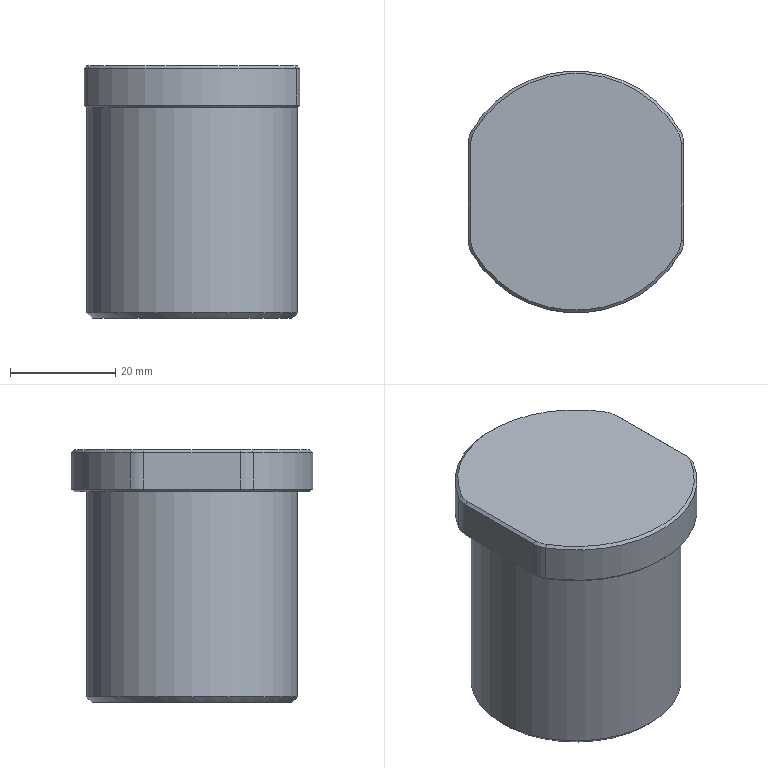Part | STEP file | lll_id150_x_t | 1 solid | 32 faces | box 41 x 46 x 48 mm | volume 57755 mm3 | cone 14 | plane 10 | cylinder 8 | commonest cylinder face diameters 10 x4 46 x2 14 x1 40 x1
STEP:
#1=CARTESIAN_POINT('',(-19.375,11.439,-143.5));
#2=VERTEX_POINT('',#1);
#3=CARTESIAN_POINT('',(19.375,11.439,-143.5));
#4=VERTEX_POINT('',#3);
#5=CARTESIAN_POINT('',(0.,0.,-143.5));
#6=DIRECTION('',(0.,0.,-1.));
#7=DIRECTION('',(-1.,0.,0.));
#8=AXIS2_PLACEMENT_3D('',#5,#6,#7);
#9=CIRCLE('',#8,22.5);
#10=EDGE_CURVE('',#2,#4,#9,.T.);
#11=ORIENTED_EDGE('',*,*,#10,.T.);
#12=CARTESIAN_POINT('',(20.,9.152,-143.5));
#13=VERTEX_POINT('',#12);
#14=CARTESIAN_POINT('',(15.5,9.152,-143.5));
#15=DIRECTION('',(0.,0.,-1.));
#16=DIRECTION('',(-1.,0.,0.));
#17=AXIS2_PLACEMENT_3D('',#14,#15,#16);
#18=CIRCLE('',#17,4.5);
#19=EDGE_CURVE('',#4,#13,#18,.T.);
#20=ORIENTED_EDGE('',*,*,#19,.T.);
#21=CARTESIAN_POINT('',(20.,0.,-143.5));
#22=VERTEX_POINT('',#21);
#23=CARTESIAN_POINT('',(20.,0.,-143.5));
#24=DIRECTION('',(0.,-1.,0.));
#25=VECTOR('',#24,1.);
#26=LINE('',#23,#25);
#27=EDGE_CURVE('',#13,#22,#26,.T.);
#28=ORIENTED_EDGE('',*,*,#27,.T.);
#29=CARTESIAN_POINT('',(-20.,0.,-143.5));
#30=VERTEX_POINT('',#29);
#31=CARTESIAN_POINT('',(0.,0.,-143.5));
#32=DIRECTION('',(0.,0.,1.));
#33=DIRECTION('',(1.,0.,0.));
#34=AXIS2_PLACEMENT_3D('',#31,#32,#33);
#35=CIRCLE('',#34,20.);
#36=EDGE_CURVE('',#22,#30,#35,.T.);
#37=ORIENTED_EDGE('',*,*,#36,.T.);
#38=CARTESIAN_POINT('',(-20.,9.152,-143.5));
#39=VERTEX_POINT('',#38);
#40=CARTESIAN_POINT('',(-20.,9.152,-143.5));
#41=DIRECTION('',(0.,1.,0.));
#42=VECTOR('',#41,1.);
#43=LINE('',#40,#42);
#44=EDGE_CURVE('',#30,#39,#43,.T.);
#45=ORIENTED_EDGE('',*,*,#44,.T.);
#46=CARTESIAN_POINT('',(-15.5,9.152,-143.5));
#47=DIRECTION('',(0.,0.,-1.));
#48=DIRECTION('',(-1.,0.,0.));
#49=AXIS2_PLACEMENT_3D('',#46,#47,#48);
#50=CIRCLE('',#49,4.5);
#51=EDGE_CURVE('',#39,#2,#50,.T.);
#52=ORIENTED_EDGE('',*,*,#51,.T.);
#53=EDGE_LOOP('',(#11,#20,#28,#37,#45,#52));
#54=FACE_OUTER_BOUND('',#53,.T.);
#55=CARTESIAN_POINT('',(0.,0.,-143.5));
#56=DIRECTION('',(0.,0.,-1.));
#57=DIRECTION('',(-1.,0.,0.));
#58=AXIS2_PLACEMENT_3D('',#55,#56,#57);
#59=PLANE('',#58);
#60=ADVANCED_FACE('',(#54),#59,.T.);
#61=CARTESIAN_POINT('',(-19.806,11.694,-136.));
#62=VERTEX_POINT('',#61);
#63=CARTESIAN_POINT('',(19.806,11.694,-136.));
#64=VERTEX_POINT('',#63);
#65=CARTESIAN_POINT('',(0.,0.,-136.));
#66=DIRECTION('',(0.,0.,-1.));
#67=DIRECTION('',(1.,0.,0.));
#68=AXIS2_PLACEMENT_3D('',#65,#66,#67);
#69=CIRCLE('',#68,23.);
#70=EDGE_CURVE('',#62,#64,#69,.T.);
#71=ORIENTED_EDGE('',*,*,#70,.T.);
#72=CARTESIAN_POINT('',(19.806,11.694,-143.));
#73=VERTEX_POINT('',#72);
#74=CARTESIAN_POINT('',(19.806,11.694,-143.5));
#75=DIRECTION('',(0.,0.,-1.));
#76=VECTOR('',#75,1.);
#77=LINE('',#74,#76);
#78=EDGE_CURVE('',#64,#73,#77,.T.);
#79=ORIENTED_EDGE('',*,*,#78,.T.);
#80=CARTESIAN_POINT('',(-19.806,11.694,-143.));
#81=VERTEX_POINT('',#80);
#82=CARTESIAN_POINT('',(0.,0.,-143.));
#83=DIRECTION('',(0.,0.,1.));
#84=DIRECTION('',(-1.,0.,0.));
#85=AXIS2_PLACEMENT_3D('',#82,#83,#84);
#86=CIRCLE('',#85,23.);
#87=EDGE_CURVE('',#73,#81,#86,.T.);
#88=ORIENTED_EDGE('',*,*,#87,.T.);
#89=CARTESIAN_POINT('',(-19.806,11.694,-143.5));
#90=DIRECTION('',(0.,0.,1.));
#91=VECTOR('',#90,1.);
#92=LINE('',#89,#91);
#93=EDGE_CURVE('',#81,#62,#92,.T.);
#94=ORIENTED_EDGE('',*,*,#93,.T.);
#95=EDGE_LOOP('',(#71,#79,#88,#94));
#96=FACE_OUTER_BOUND('',#95,.T.);
#97=CARTESIAN_POINT('',(0.,0.,-143.5));
#98=DIRECTION('',(0.,0.,1.));
#99=DIRECTION('',(1.,0.,0.));
#100=AXIS2_PLACEMENT_3D('',#97,#98,#99);
#101=CYLINDRICAL_SURFACE('',#100,23.);
#102=ADVANCED_FACE('',(#96),#101,.T.);
#103=CARTESIAN_POINT('',(20.,-9.152,-143.5));
#104=VERTEX_POINT('',#103);
#105=CARTESIAN_POINT('',(20.,0.,-143.5));
#106=DIRECTION('',(0.,-1.,0.));
#107=VECTOR('',#106,1.);
#108=LINE('',#105,#107);
#109=EDGE_CURVE('',#22,#104,#108,.T.);
#110=ORIENTED_EDGE('',*,*,#109,.T.);
#111=CARTESIAN_POINT('',(19.375,-11.439,-143.5));
#112=VERTEX_POINT('',#111);
#113=CARTESIAN_POINT('',(15.5,-9.152,-143.5));
#114=DIRECTION('',(0.,0.,-1.));
#115=DIRECTION('',(-1.,0.,0.));
#116=AXIS2_PLACEMENT_3D('',#113,#114,#115);
#117=CIRCLE('',#116,4.5);
#118=EDGE_CURVE('',#104,#112,#117,.T.);
#119=ORIENTED_EDGE('',*,*,#118,.T.);
#120=CARTESIAN_POINT('',(-19.375,-11.439,-143.5));
#121=VERTEX_POINT('',#120);
#122=CARTESIAN_POINT('',(0.,0.,-143.5));
#123=DIRECTION('',(0.,0.,-1.));
#124=DIRECTION('',(-1.,0.,0.));
#125=AXIS2_PLACEMENT_3D('',#122,#123,#124);
#126=CIRCLE('',#125,22.5);
#127=EDGE_CURVE('',#112,#121,#126,.T.);
#128=ORIENTED_EDGE('',*,*,#127,.T.);
#129=CARTESIAN_POINT('',(-20.,-9.152,-143.5));
#130=VERTEX_POINT('',#129);
#131=CARTESIAN_POINT('',(-15.5,-9.152,-143.5));
#132=DIRECTION('',(0.,0.,-1.));
#133=DIRECTION('',(-1.,0.,0.));
#134=AXIS2_PLACEMENT_3D('',#131,#132,#133);
#135=CIRCLE('',#134,4.5);
#136=EDGE_CURVE('',#121,#130,#135,.T.);
#137=ORIENTED_EDGE('',*,*,#136,.T.);
#138=CARTESIAN_POINT('',(-20.,9.152,-143.5));
#139=DIRECTION('',(0.,1.,0.));
#140=VECTOR('',#139,1.);
#141=LINE('',#138,#140);
#142=EDGE_CURVE('',#130,#30,#141,.T.);
#143=ORIENTED_EDGE('',*,*,#142,.T.);
#144=CARTESIAN_POINT('',(0.,0.,-143.5));
#145=DIRECTION('',(0.,0.,1.));
#146=DIRECTION('',(1.,0.,0.));
#147=AXIS2_PLACEMENT_3D('',#144,#145,#146);
#148=CIRCLE('',#147,20.);
#149=EDGE_CURVE('',#30,#22,#148,.T.);
#150=ORIENTED_EDGE('',*,*,#149,.T.);
#151=EDGE_LOOP('',(#110,#119,#128,#137,#143,#150));
#152=FACE_OUTER_BOUND('',#151,.T.);
#153=CARTESIAN_POINT('',(0.,0.,-143.5));
#154=DIRECTION('',(0.,0.,-1.));
#155=DIRECTION('',(-1.,0.,0.));
#156=AXIS2_PLACEMENT_3D('',#153,#154,#155);
#157=PLANE('',#156);
#158=ADVANCED_FACE('',(#152),#157,.T.);
#159=CARTESIAN_POINT('',(-20.,9.152,-135.5));
#160=VERTEX_POINT('',#159);
#161=CARTESIAN_POINT('',(-20.,-9.152,-135.5));
#162=VERTEX_POINT('',#161);
#163=CARTESIAN_POINT('',(-20.,-9.152,-135.5));
#164=DIRECTION('',(0.,-1.,0.));
#165=VECTOR('',#164,1.);
#166=LINE('',#163,#165);
#167=EDGE_CURVE('',#160,#162,#166,.T.);
#168=ORIENTED_EDGE('',*,*,#167,.T.);
#169=CARTESIAN_POINT('',(-19.375,-11.439,-135.5));
#170=VERTEX_POINT('',#169);
#171=CARTESIAN_POINT('',(-15.5,-9.152,-135.5));
#172=DIRECTION('',(0.,0.,1.));
#173=DIRECTION('',(1.,0.,0.));
#174=AXIS2_PLACEMENT_3D('',#171,#172,#173);
#175=CIRCLE('',#174,4.5);
#176=EDGE_CURVE('',#162,#170,#175,.T.);
#177=ORIENTED_EDGE('',*,*,#176,.T.);
#178=CARTESIAN_POINT('',(19.375,-11.439,-135.5));
#179=VERTEX_POINT('',#178);
#180=CARTESIAN_POINT('',(0.,0.,-135.5));
#181=DIRECTION('',(0.,0.,1.));
#182=DIRECTION('',(1.,0.,0.));
#183=AXIS2_PLACEMENT_3D('',#180,#181,#182);
#184=CIRCLE('',#183,22.5);
#185=EDGE_CURVE('',#170,#179,#184,.T.);
#186=ORIENTED_EDGE('',*,*,#185,.T.);
#187=CARTESIAN_POINT('',(20.,-9.152,-135.5));
#188=VERTEX_POINT('',#187);
#189=CARTESIAN_POINT('',(15.5,-9.152,-135.5));
#190=DIRECTION('',(0.,0.,1.));
#191=DIRECTION('',(1.,0.,0.));
#192=AXIS2_PLACEMENT_3D('',#189,#190,#191);
#193=CIRCLE('',#192,4.5);
#194=EDGE_CURVE('',#179,#188,#193,.T.);
#195=ORIENTED_EDGE('',*,*,#194,.T.);
#196=CARTESIAN_POINT('',(20.,9.152,-135.5));
#197=VERTEX_POINT('',#196);
#198=CARTESIAN_POINT('',(20.,0.,-135.5));
#199=DIRECTION('',(0.,1.,0.));
#200=VECTOR('',#199,1.);
#201=LINE('',#198,#200);
#202=EDGE_CURVE('',#188,#197,#201,.T.);
#203=ORIENTED_EDGE('',*,*,#202,.T.);
#204=CARTESIAN_POINT('',(19.375,11.439,-135.5));
#205=VERTEX_POINT('',#204);
#206=CARTESIAN_POINT('',(15.5,9.152,-135.5));
#207=DIRECTION('',(0.,0.,1.));
#208=DIRECTION('',(1.,0.,0.));
#209=AXIS2_PLACEMENT_3D('',#206,#207,#208);
#210=CIRCLE('',#209,4.5);
#211=EDGE_CURVE('',#197,#205,#210,.T.);
#212=ORIENTED_EDGE('',*,*,#211,.T.);
#213=CARTESIAN_POINT('',(-19.375,11.439,-135.5));
#214=VERTEX_POINT('',#213);
#215=CARTESIAN_POINT('',(0.,0.,-135.5));
#216=DIRECTION('',(0.,0.,1.));
#217=DIRECTION('',(1.,0.,0.));
#218=AXIS2_PLACEMENT_3D('',#215,#216,#217);
#219=CIRCLE('',#218,22.5);
#220=EDGE_CURVE('',#205,#214,#219,.T.);
#221=ORIENTED_EDGE('',*,*,#220,.T.);
#222=CARTESIAN_POINT('',(-15.5,9.152,-135.5));
#223=DIRECTION('',(0.,0.,1.));
#224=DIRECTION('',(1.,0.,0.));
#225=AXIS2_PLACEMENT_3D('',#222,#223,#224);
#226=CIRCLE('',#225,4.5);
#227=EDGE_CURVE('',#214,#160,#226,.T.);
#228=ORIENTED_EDGE('',*,*,#227,.T.);
#229=EDGE_LOOP('',(#168,#177,#186,#195,#203,#212,#221,#228));
#230=FACE_OUTER_BOUND('',#229,.T.);
#231=CARTESIAN_POINT('',(0.,0.,-135.5));
#232=DIRECTION('',(0.,0.,1.));
#233=DIRECTION('',(1.,0.,0.));
#234=AXIS2_PLACEMENT_3D('',#231,#232,#233);
#235=PLANE('',#234);
#236=ADVANCED_FACE('',(#230),#235,.T.);
#237=CARTESIAN_POINT('',(-19.806,-11.694,-143.));
#238=VERTEX_POINT('',#237);
#239=CARTESIAN_POINT('',(19.806,-11.694,-143.));
#240=VERTEX_POINT('',#239);
#241=CARTESIAN_POINT('',(0.,0.,-143.));
#242=DIRECTION('',(0.,0.,1.));
#243=DIRECTION('',(-1.,0.,0.));
#244=AXIS2_PLACEMENT_3D('',#241,#242,#243);
#245=CIRCLE('',#244,23.);
#246=EDGE_CURVE('',#238,#240,#245,.T.);
#247=ORIENTED_EDGE('',*,*,#246,.T.);
#248=CARTESIAN_POINT('',(19.806,-11.694,-136.));
#249=VERTEX_POINT('',#248);
#250=CARTESIAN_POINT('',(19.806,-11.694,-143.5));
#251=DIRECTION('',(0.,0.,1.));
#252=VECTOR('',#251,1.);
#253=LINE('',#250,#252);
#254=EDGE_CURVE('',#240,#249,#253,.T.);
#255=ORIENTED_EDGE('',*,*,#254,.T.);
#256=CARTESIAN_POINT('',(-19.806,-11.694,-136.));
#257=VERTEX_POINT('',#256);
#258=CARTESIAN_POINT('',(0.,0.,-136.));
#259=DIRECTION('',(0.,0.,-1.));
#260=DIRECTION('',(1.,0.,0.));
#261=AXIS2_PLACEMENT_3D('',#258,#259,#260);
#262=CIRCLE('',#261,23.);
#263=EDGE_CURVE('',#249,#257,#262,.T.);
#264=ORIENTED_EDGE('',*,*,#263,.T.);
#265=CARTESIAN_POINT('',(-19.806,-11.694,-143.5));
#266=DIRECTION('',(0.,0.,-1.));
#267=VECTOR('',#266,1.);
#268=LINE('',#265,#267);
#269=EDGE_CURVE('',#257,#238,#268,.T.);
#270=ORIENTED_EDGE('',*,*,#269,.T.);
#271=EDGE_LOOP('',(#247,#255,#264,#270));
#272=FACE_OUTER_BOUND('',#271,.T.);
#273=CARTESIAN_POINT('',(0.,0.,-143.5));
#274=DIRECTION('',(0.,0.,1.));
#275=DIRECTION('',(1.,0.,0.));
#276=AXIS2_PLACEMENT_3D('',#273,#274,#275);
#277=CYLINDRICAL_SURFACE('',#276,23.);
#278=ADVANCED_FACE('',(#272),#277,.T.);
#279=CARTESIAN_POINT('',(20.,0.,-182.5));
#280=VERTEX_POINT('',#279);
#281=CARTESIAN_POINT('',(0.,0.,-182.5));
#282=DIRECTION('',(0.,0.,1.));
#283=DIRECTION('',(1.,0.,0.));
#284=AXIS2_PLACEMENT_3D('',#281,#282,#283);
#285=CIRCLE('',#284,20.);
#286=EDGE_CURVE('',#280,#280,#285,.T.);
#287=ORIENTED_EDGE('',*,*,#286,.T.);
#288=EDGE_LOOP('',(#287));
#289=FACE_BOUND('',#288,.T.);
#290=ORIENTED_EDGE('',*,*,#149,.F.);
#291=ORIENTED_EDGE('',*,*,#36,.F.);
#292=EDGE_LOOP('',(#290,#291));
#293=FACE_BOUND('',#292,.T.);
#294=CARTESIAN_POINT('',(0.,0.,-183.5));
#295=DIRECTION('',(0.,0.,1.));
#296=DIRECTION('',(1.,0.,0.));
#297=AXIS2_PLACEMENT_3D('',#294,#295,#296);
#298=CYLINDRICAL_SURFACE('',#297,20.);
#299=ADVANCED_FACE('',(#289,#293),#298,.T.);
#300=CARTESIAN_POINT('',(7.,0.,-183.5));
#301=VERTEX_POINT('',#300);
#302=CARTESIAN_POINT('',(0.,0.,-183.5));
#303=DIRECTION('',(0.,0.,1.));
#304=DIRECTION('',(1.,0.,0.));
#305=AXIS2_PLACEMENT_3D('',#302,#303,#304);
#306=CIRCLE('',#305,7.);
#307=EDGE_CURVE('',#301,#301,#306,.T.);
#308=ORIENTED_EDGE('',*,*,#307,.T.);
#309=EDGE_LOOP('',(#308));
#310=FACE_BOUND('',#309,.T.);
#311=CARTESIAN_POINT('',(19.,0.,-183.5));
#312=VERTEX_POINT('',#311);
#313=CARTESIAN_POINT('',(0.,0.,-183.5));
#314=DIRECTION('',(0.,0.,-1.));
#315=DIRECTION('',(1.,0.,0.));
#316=AXIS2_PLACEMENT_3D('',#313,#314,#315);
#317=CIRCLE('',#316,19.);
#318=EDGE_CURVE('',#312,#312,#317,.T.);
#319=ORIENTED_EDGE('',*,*,#318,.T.);
#320=EDGE_LOOP('',(#319));
#321=FACE_BOUND('',#320,.T.);
#322=CARTESIAN_POINT('',(0.,0.,-183.5));
#323=DIRECTION('',(0.,0.,1.));
#324=DIRECTION('',(1.,0.,0.));
#325=AXIS2_PLACEMENT_3D('',#322,#323,#324);
#326=PLANE('',#325);
#327=ADVANCED_FACE('',(#310,#321),#326,.F.);
#328=CARTESIAN_POINT('',(20.5,-9.152,-136.));
#329=VERTEX_POINT('',#328);
#330=CARTESIAN_POINT('',(20.5,-9.152,-143.));
#331=VERTEX_POINT('',#330);
#332=CARTESIAN_POINT('',(20.5,-9.152,-143.5));
#333=DIRECTION('',(0.,0.,-1.));
#334=VECTOR('',#333,1.);
#335=LINE('',#332,#334);
#336=EDGE_CURVE('',#329,#331,#335,.T.);
#337=ORIENTED_EDGE('',*,*,#336,.T.);
#338=CARTESIAN_POINT('',(20.5,9.152,-143.));
#339=VERTEX_POINT('',#338);
#340=CARTESIAN_POINT('',(20.5,0.,-143.));
#341=DIRECTION('',(0.,1.,0.));
#342=VECTOR('',#341,1.);
#343=LINE('',#340,#342);
#344=EDGE_CURVE('',#331,#339,#343,.T.);
#345=ORIENTED_EDGE('',*,*,#344,.T.);
#346=CARTESIAN_POINT('',(20.5,9.152,-136.));
#347=VERTEX_POINT('',#346);
#348=CARTESIAN_POINT('',(20.5,9.152,-143.5));
#349=DIRECTION('',(0.,0.,1.));
#350=VECTOR('',#349,1.);
#351=LINE('',#348,#350);
#352=EDGE_CURVE('',#339,#347,#351,.T.);
#353=ORIENTED_EDGE('',*,*,#352,.T.);
#354=CARTESIAN_POINT('',(20.5,0.,-136.));
#355=DIRECTION('',(0.,-1.,0.));
#356=VECTOR('',#355,1.);
#357=LINE('',#354,#356);
#358=EDGE_CURVE('',#347,#329,#357,.T.);
#359=ORIENTED_EDGE('',*,*,#358,.T.);
#360=EDGE_LOOP('',(#337,#345,#353,#359));
#361=FACE_OUTER_BOUND('',#360,.T.);
#362=CARTESIAN_POINT('',(20.5,0.,-143.5));
#363=DIRECTION('',(1.,0.,0.));
#364=DIRECTION('',(0.,0.,-1.));
#365=AXIS2_PLACEMENT_3D('',#362,#363,#364);
#366=PLANE('',#365);
#367=ADVANCED_FACE('',(#361),#366,.T.);
#368=CARTESIAN_POINT('',(-20.5,9.152,-136.));
#369=VERTEX_POINT('',#368);
#370=CARTESIAN_POINT('',(-20.5,9.152,-143.));
#371=VERTEX_POINT('',#370);
#372=CARTESIAN_POINT('',(-20.5,9.152,-143.));
#373=DIRECTION('',(0.,0.,-1.));
#374=VECTOR('',#373,1.);
#375=LINE('',#372,#374);
#376=EDGE_CURVE('',#369,#371,#375,.T.);
#377=ORIENTED_EDGE('',*,*,#376,.T.);
#378=CARTESIAN_POINT('',(-20.5,-9.152,-143.));
#379=VERTEX_POINT('',#378);
#380=CARTESIAN_POINT('',(-20.5,-9.152,-143.));
#381=DIRECTION('',(0.,-1.,0.));
#382=VECTOR('',#381,1.);
#383=LINE('',#380,#382);
#384=EDGE_CURVE('',#371,#379,#383,.T.);
#385=ORIENTED_EDGE('',*,*,#384,.T.);
#386=CARTESIAN_POINT('',(-20.5,-9.152,-136.));
#387=VERTEX_POINT('',#386);
#388=CARTESIAN_POINT('',(-20.5,-9.152,-136.));
#389=DIRECTION('',(0.,0.,1.));
#390=VECTOR('',#389,1.);
#391=LINE('',#388,#390);
#392=EDGE_CURVE('',#379,#387,#391,.T.);
#393=ORIENTED_EDGE('',*,*,#392,.T.);
#394=CARTESIAN_POINT('',(-20.5,9.152,-136.));
#395=DIRECTION('',(0.,1.,0.));
#396=VECTOR('',#395,1.);
#397=LINE('',#394,#396);
#398=EDGE_CURVE('',#387,#369,#397,.T.);
#399=ORIENTED_EDGE('',*,*,#398,.T.);
#400=EDGE_LOOP('',(#377,#385,#393,#399));
#401=FACE_OUTER_BOUND('',#400,.T.);
#402=CARTESIAN_POINT('',(-20.5,0.,-143.5));
#403=DIRECTION('',(1.,0.,0.));
#404=DIRECTION('',(0.,0.,-1.));
#405=AXIS2_PLACEMENT_3D('',#402,#403,#404);
#406=PLANE('',#405);
#407=ADVANCED_FACE('',(#401),#406,.F.);
#408=ORIENTED_EDGE('',*,*,#70,.F.);
#409=CARTESIAN_POINT('',(-15.5,9.152,-131.));
#410=DIRECTION('',(0.6089,-0.3595,0.7071));
#411=VECTOR('',#410,1.);
#412=LINE('',#409,#411);
#413=EDGE_CURVE('',#62,#214,#412,.T.);
#414=ORIENTED_EDGE('',*,*,#413,.T.);
#415=ORIENTED_EDGE('',*,*,#220,.F.);
#416=CARTESIAN_POINT('',(15.5,9.152,-131.));
#417=DIRECTION('',(0.6089,0.3595,-0.7071));
#418=VECTOR('',#417,1.);
#419=LINE('',#416,#418);
#420=EDGE_CURVE('',#205,#64,#419,.T.);
#421=ORIENTED_EDGE('',*,*,#420,.T.);
#422=EDGE_LOOP('',(#408,#414,#415,#421));
#423=FACE_OUTER_BOUND('',#422,.T.);
#424=CARTESIAN_POINT('',(0.,0.,-136.));
#425=DIRECTION('',(0.,0.,-1.));
#426=DIRECTION('',(-1.,0.,0.));
#427=AXIS2_PLACEMENT_3D('',#424,#425,#426);
#428=CONICAL_SURFACE('',#427,23.,45.);
#429=ADVANCED_FACE('',(#423),#428,.T.);
#430=ORIENTED_EDGE('',*,*,#87,.F.);
#431=CARTESIAN_POINT('',(15.5,9.152,-148.));
#432=DIRECTION('',(-0.6089,-0.3595,-0.7071));
#433=VECTOR('',#432,1.);
#434=LINE('',#431,#433);
#435=EDGE_CURVE('',#73,#4,#434,.T.);
#436=ORIENTED_EDGE('',*,*,#435,.T.);
#437=ORIENTED_EDGE('',*,*,#10,.F.);
#438=CARTESIAN_POINT('',(-15.5,9.152,-148.));
#439=DIRECTION('',(-0.6089,0.3595,0.7071));
#440=VECTOR('',#439,1.);
#441=LINE('',#438,#440);
#442=EDGE_CURVE('',#2,#81,#441,.T.);
#443=ORIENTED_EDGE('',*,*,#442,.T.);
#444=EDGE_LOOP('',(#430,#436,#437,#443));
#445=FACE_OUTER_BOUND('',#444,.T.);
#446=CARTESIAN_POINT('',(0.,0.,-143.));
#447=DIRECTION('',(0.,0.,1.));
#448=DIRECTION('',(1.,0.,0.));
#449=AXIS2_PLACEMENT_3D('',#446,#447,#448);
#450=CONICAL_SURFACE('',#449,23.,45.);
#451=ADVANCED_FACE('',(#445),#450,.T.);
#452=ORIENTED_EDGE('',*,*,#185,.F.);
#453=CARTESIAN_POINT('',(-15.5,-9.152,-131.));
#454=DIRECTION('',(-0.6089,-0.3595,-0.7071));
#455=VECTOR('',#454,1.);
#456=LINE('',#453,#455);
#457=EDGE_CURVE('',#170,#257,#456,.T.);
#458=ORIENTED_EDGE('',*,*,#457,.T.);
#459=ORIENTED_EDGE('',*,*,#263,.F.);
#460=CARTESIAN_POINT('',(15.5,-9.152,-131.));
#461=DIRECTION('',(-0.6089,0.3595,0.7071));
#462=VECTOR('',#461,1.);
#463=LINE('',#460,#462);
#464=EDGE_CURVE('',#249,#179,#463,.T.);
#465=ORIENTED_EDGE('',*,*,#464,.T.);
#466=EDGE_LOOP('',(#452,#458,#459,#465));
#467=FACE_OUTER_BOUND('',#466,.T.);
#468=CARTESIAN_POINT('',(0.,0.,-136.));
#469=DIRECTION('',(0.,0.,-1.));
#470=DIRECTION('',(-1.,0.,0.));
#471=AXIS2_PLACEMENT_3D('',#468,#469,#470);
#472=CONICAL_SURFACE('',#471,23.,45.);
#473=ADVANCED_FACE('',(#467),#472,.T.);
#474=ORIENTED_EDGE('',*,*,#127,.F.);
#475=CARTESIAN_POINT('',(15.5,-9.152,-148.));
#476=DIRECTION('',(0.6089,-0.3595,0.7071));
#477=VECTOR('',#476,1.);
#478=LINE('',#475,#477);
#479=EDGE_CURVE('',#112,#240,#478,.T.);
#480=ORIENTED_EDGE('',*,*,#479,.T.);
#481=ORIENTED_EDGE('',*,*,#246,.F.);
#482=CARTESIAN_POINT('',(-15.5,-9.152,-148.));
#483=DIRECTION('',(0.6089,0.3595,-0.7071));
#484=VECTOR('',#483,1.);
#485=LINE('',#482,#484);
#486=EDGE_CURVE('',#238,#121,#485,.T.);
#487=ORIENTED_EDGE('',*,*,#486,.T.);
#488=EDGE_LOOP('',(#474,#480,#481,#487));
#489=FACE_OUTER_BOUND('',#488,.T.);
#490=CARTESIAN_POINT('',(0.,0.,-143.));
#491=DIRECTION('',(0.,0.,1.));
#492=DIRECTION('',(1.,0.,0.));
#493=AXIS2_PLACEMENT_3D('',#490,#491,#492);
#494=CONICAL_SURFACE('',#493,23.,45.);
#495=ADVANCED_FACE('',(#489),#494,.T.);
#496=ORIENTED_EDGE('',*,*,#318,.F.);
#497=EDGE_LOOP('',(#496));
#498=FACE_BOUND('',#497,.T.);
#499=ORIENTED_EDGE('',*,*,#286,.F.);
#500=EDGE_LOOP('',(#499));
#501=FACE_BOUND('',#500,.T.);
#502=CARTESIAN_POINT('',(0.,0.,-182.5));
#503=DIRECTION('',(0.,0.,1.));
#504=DIRECTION('',(1.,0.,0.));
#505=AXIS2_PLACEMENT_3D('',#502,#503,#504);
#506=CONICAL_SURFACE('',#505,20.,45.);
#507=ADVANCED_FACE('',(#498,#501),#506,.T.);
#508=CARTESIAN_POINT('',(7.,0.,-151.5));
#509=VERTEX_POINT('',#508);
#510=CARTESIAN_POINT('',(0.,0.,-151.5));
#511=DIRECTION('',(0.,0.,1.));
#512=DIRECTION('',(1.,0.,0.));
#513=AXIS2_PLACEMENT_3D('',#510,#511,#512);
#514=CIRCLE('',#513,7.);
#515=EDGE_CURVE('',#509,#509,#514,.T.);
#516=ORIENTED_EDGE('',*,*,#515,.F.);
#517=EDGE_LOOP('',(#516));
#518=FACE_BOUND('',#517,.T.);
#519=CARTESIAN_POINT('',(0.,0.,-147.294));
#520=VERTEX_POINT('',#519);
#521=VERTEX_LOOP('',#520);
#522=FACE_BOUND('',#521,.T.);
#523=CARTESIAN_POINT('',(0.,0.,-151.5));
#524=DIRECTION('',(0.,0.,-1.));
#525=DIRECTION('',(-1.,0.,0.));
#526=AXIS2_PLACEMENT_3D('',#523,#524,#525);
#527=CONICAL_SURFACE('',#526,7.,59.);
#528=ADVANCED_FACE('',(#518,#522),#527,.F.);
#529=ORIENTED_EDGE('',*,*,#515,.T.);
#530=EDGE_LOOP('',(#529));
#531=FACE_BOUND('',#530,.T.);
#532=ORIENTED_EDGE('',*,*,#307,.F.);
#533=EDGE_LOOP('',(#532));
#534=FACE_BOUND('',#533,.T.);
#535=CARTESIAN_POINT('',(0.,0.,-183.5));
#536=DIRECTION('',(0.,0.,1.));
#537=DIRECTION('',(1.,0.,0.));
#538=AXIS2_PLACEMENT_3D('',#535,#536,#537);
#539=CYLINDRICAL_SURFACE('',#538,7.);
#540=ADVANCED_FACE('',(#531,#534),#539,.F.);
#541=ORIENTED_EDGE('',*,*,#352,.F.);
#542=CARTESIAN_POINT('',(15.5,9.152,-143.));
#543=DIRECTION('',(0.,0.,1.));
#544=DIRECTION('',(-1.,0.,0.));
#545=AXIS2_PLACEMENT_3D('',#542,#543,#544);
#546=CIRCLE('',#545,5.);
#547=EDGE_CURVE('',#339,#73,#546,.T.);
#548=ORIENTED_EDGE('',*,*,#547,.T.);
#549=ORIENTED_EDGE('',*,*,#78,.F.);
#550=CARTESIAN_POINT('',(15.5,9.152,-136.));
#551=DIRECTION('',(0.,0.,-1.));
#552=DIRECTION('',(1.,0.,0.));
#553=AXIS2_PLACEMENT_3D('',#550,#551,#552);
#554=CIRCLE('',#553,5.);
#555=EDGE_CURVE('',#64,#347,#554,.T.);
#556=ORIENTED_EDGE('',*,*,#555,.T.);
#557=EDGE_LOOP('',(#541,#548,#549,#556));
#558=FACE_OUTER_BOUND('',#557,.T.);
#559=CARTESIAN_POINT('',(15.5,9.152,-143.5));
#560=DIRECTION('',(0.,0.,1.));
#561=DIRECTION('',(1.,0.,0.));
#562=AXIS2_PLACEMENT_3D('',#559,#560,#561);
#563=CYLINDRICAL_SURFACE('',#562,5.);
#564=ADVANCED_FACE('',(#558),#563,.T.);
#565=ORIENTED_EDGE('',*,*,#254,.F.);
#566=CARTESIAN_POINT('',(15.5,-9.152,-143.));
#567=DIRECTION('',(0.,0.,1.));
#568=DIRECTION('',(-1.,0.,0.));
#569=AXIS2_PLACEMENT_3D('',#566,#567,#568);
#570=CIRCLE('',#569,5.);
#571=EDGE_CURVE('',#240,#331,#570,.T.);
#572=ORIENTED_EDGE('',*,*,#571,.T.);
#573=ORIENTED_EDGE('',*,*,#336,.F.);
#574=CARTESIAN_POINT('',(15.5,-9.152,-136.));
#575=DIRECTION('',(0.,0.,-1.));
#576=DIRECTION('',(1.,0.,0.));
#577=AXIS2_PLACEMENT_3D('',#574,#575,#576);
#578=CIRCLE('',#577,5.);
#579=EDGE_CURVE('',#329,#249,#578,.T.);
#580=ORIENTED_EDGE('',*,*,#579,.T.);
#581=EDGE_LOOP('',(#565,#572,#573,#580));
#582=FACE_OUTER_BOUND('',#581,.T.);
#583=CARTESIAN_POINT('',(15.5,-9.152,-143.5));
#584=DIRECTION('',(0.,0.,1.));
#585=DIRECTION('',(1.,0.,0.));
#586=AXIS2_PLACEMENT_3D('',#583,#584,#585);
#587=CYLINDRICAL_SURFACE('',#586,5.);
#588=ADVANCED_FACE('',(#582),#587,.T.);
#589=ORIENTED_EDGE('',*,*,#93,.F.);
#590=CARTESIAN_POINT('',(-15.5,9.152,-143.));
#591=DIRECTION('',(0.,0.,1.));
#592=DIRECTION('',(-1.,0.,0.));
#593=AXIS2_PLACEMENT_3D('',#590,#591,#592);
#594=CIRCLE('',#593,5.);
#595=EDGE_CURVE('',#81,#371,#594,.T.);
#596=ORIENTED_EDGE('',*,*,#595,.T.);
#597=ORIENTED_EDGE('',*,*,#376,.F.);
#598=CARTESIAN_POINT('',(-15.5,9.152,-136.));
#599=DIRECTION('',(0.,0.,-1.));
#600=DIRECTION('',(1.,0.,0.));
#601=AXIS2_PLACEMENT_3D('',#598,#599,#600);
#602=CIRCLE('',#601,5.);
#603=EDGE_CURVE('',#369,#62,#602,.T.);
#604=ORIENTED_EDGE('',*,*,#603,.T.);
#605=EDGE_LOOP('',(#589,#596,#597,#604));
#606=FACE_OUTER_BOUND('',#605,.T.);
#607=CARTESIAN_POINT('',(-15.5,9.152,-143.5));
#608=DIRECTION('',(0.,0.,1.));
#609=DIRECTION('',(1.,0.,0.));
#610=AXIS2_PLACEMENT_3D('',#607,#608,#609);
#611=CYLINDRICAL_SURFACE('',#610,5.);
#612=ADVANCED_FACE('',(#606),#611,.T.);
#613=ORIENTED_EDGE('',*,*,#392,.F.);
#614=CARTESIAN_POINT('',(-15.5,-9.152,-143.));
#615=DIRECTION('',(0.,0.,1.));
#616=DIRECTION('',(-1.,0.,0.));
#617=AXIS2_PLACEMENT_3D('',#614,#615,#616);
#618=CIRCLE('',#617,5.);
#619=EDGE_CURVE('',#379,#238,#618,.T.);
#620=ORIENTED_EDGE('',*,*,#619,.T.);
#621=ORIENTED_EDGE('',*,*,#269,.F.);
#622=CARTESIAN_POINT('',(-15.5,-9.152,-136.));
#623=DIRECTION('',(0.,0.,-1.));
#624=DIRECTION('',(1.,0.,0.));
#625=AXIS2_PLACEMENT_3D('',#622,#623,#624);
#626=CIRCLE('',#625,5.);
#627=EDGE_CURVE('',#257,#387,#626,.T.);
#628=ORIENTED_EDGE('',*,*,#627,.T.);
#629=EDGE_LOOP('',(#613,#620,#621,#628));
#630=FACE_OUTER_BOUND('',#629,.T.);
#631=CARTESIAN_POINT('',(-15.5,-9.152,-143.5));
#632=DIRECTION('',(0.,0.,1.));
#633=DIRECTION('',(1.,0.,0.));
#634=AXIS2_PLACEMENT_3D('',#631,#632,#633);
#635=CYLINDRICAL_SURFACE('',#634,5.);
#636=ADVANCED_FACE('',(#630),#635,.T.);
#637=ORIENTED_EDGE('',*,*,#420,.F.);
#638=ORIENTED_EDGE('',*,*,#211,.F.);
#639=CARTESIAN_POINT('',(20.5,9.152,-136.));
#640=DIRECTION('',(-0.7071,0.,0.7071));
#641=VECTOR('',#640,1.);
#642=LINE('',#639,#641);
#643=EDGE_CURVE('',#347,#197,#642,.T.);
#644=ORIENTED_EDGE('',*,*,#643,.F.);
#645=ORIENTED_EDGE('',*,*,#555,.F.);
#646=EDGE_LOOP('',(#637,#638,#644,#645));
#647=FACE_OUTER_BOUND('',#646,.T.);
#648=CARTESIAN_POINT('',(15.5,9.152,-135.5));
#649=DIRECTION('',(0.,0.,-1.));
#650=DIRECTION('',(-1.,0.,0.));
#651=AXIS2_PLACEMENT_3D('',#648,#649,#650);
#652=CONICAL_SURFACE('',#651,4.5,45.);
#653=ADVANCED_FACE('',(#647),#652,.T.);
#654=ORIENTED_EDGE('',*,*,#643,.T.);
#655=ORIENTED_EDGE('',*,*,#202,.F.);
#656=CARTESIAN_POINT('',(20.5,-9.152,-136.));
#657=DIRECTION('',(-0.7071,0.,0.7071));
#658=VECTOR('',#657,1.);
#659=LINE('',#656,#658);
#660=EDGE_CURVE('',#329,#188,#659,.T.);
#661=ORIENTED_EDGE('',*,*,#660,.F.);
#662=ORIENTED_EDGE('',*,*,#358,.F.);
#663=EDGE_LOOP('',(#654,#655,#661,#662));
#664=FACE_OUTER_BOUND('',#663,.T.);
#665=CARTESIAN_POINT('',(20.,0.,-135.5));
#666=DIRECTION('',(-0.7071,0.,-0.7071));
#667=DIRECTION('',(-0.7071,0.,0.7071));
#668=AXIS2_PLACEMENT_3D('',#665,#666,#667);
#669=PLANE('',#668);
#670=ADVANCED_FACE('',(#664),#669,.F.);
#671=ORIENTED_EDGE('',*,*,#464,.F.);
#672=ORIENTED_EDGE('',*,*,#579,.F.);
#673=ORIENTED_EDGE('',*,*,#660,.T.);
#674=ORIENTED_EDGE('',*,*,#194,.F.);
#675=EDGE_LOOP('',(#671,#672,#673,#674));
#676=FACE_OUTER_BOUND('',#675,.T.);
#677=CARTESIAN_POINT('',(15.5,-9.152,-135.5));
#678=DIRECTION('',(0.,0.,-1.));
#679=DIRECTION('',(-1.,0.,0.));
#680=AXIS2_PLACEMENT_3D('',#677,#678,#679);
#681=CONICAL_SURFACE('',#680,4.5,45.);
#682=ADVANCED_FACE('',(#676),#681,.T.);
#683=ORIENTED_EDGE('',*,*,#486,.F.);
#684=ORIENTED_EDGE('',*,*,#619,.F.);
#685=CARTESIAN_POINT('',(-20.,-9.152,-143.5));
#686=DIRECTION('',(-0.7071,0.,0.7071));
#687=VECTOR('',#686,1.);
#688=LINE('',#685,#687);
#689=EDGE_CURVE('',#130,#379,#688,.T.);
#690=ORIENTED_EDGE('',*,*,#689,.F.);
#691=ORIENTED_EDGE('',*,*,#136,.F.);
#692=EDGE_LOOP('',(#683,#684,#690,#691));
#693=FACE_OUTER_BOUND('',#692,.T.);
#694=CARTESIAN_POINT('',(-15.5,-9.152,-143.5));
#695=DIRECTION('',(0.,0.,1.));
#696=DIRECTION('',(1.,0.,0.));
#697=AXIS2_PLACEMENT_3D('',#694,#695,#696);
#698=CONICAL_SURFACE('',#697,4.5,45.);
#699=ADVANCED_FACE('',(#693),#698,.T.);
#700=ORIENTED_EDGE('',*,*,#689,.T.);
#701=ORIENTED_EDGE('',*,*,#384,.F.);
#702=CARTESIAN_POINT('',(-20.,9.152,-143.5));
#703=DIRECTION('',(-0.7071,0.,0.7071));
#704=VECTOR('',#703,1.);
#705=LINE('',#702,#704);
#706=EDGE_CURVE('',#39,#371,#705,.T.);
#707=ORIENTED_EDGE('',*,*,#706,.F.);
#708=ORIENTED_EDGE('',*,*,#44,.F.);
#709=ORIENTED_EDGE('',*,*,#142,.F.);
#710=EDGE_LOOP('',(#700,#701,#707,#708,#709));
#711=FACE_OUTER_BOUND('',#710,.T.);
#712=CARTESIAN_POINT('',(-20.5,0.,-143.));
#713=DIRECTION('',(-0.7071,0.,-0.7071));
#714=DIRECTION('',(-0.7071,0.,0.7071));
#715=AXIS2_PLACEMENT_3D('',#712,#713,#714);
#716=PLANE('',#715);
#717=ADVANCED_FACE('',(#711),#716,.T.);
#718=ORIENTED_EDGE('',*,*,#706,.T.);
#719=ORIENTED_EDGE('',*,*,#595,.F.);
#720=ORIENTED_EDGE('',*,*,#442,.F.);
#721=ORIENTED_EDGE('',*,*,#51,.F.);
#722=EDGE_LOOP('',(#718,#719,#720,#721));
#723=FACE_OUTER_BOUND('',#722,.T.);
#724=CARTESIAN_POINT('',(-15.5,9.152,-143.5));
#725=DIRECTION('',(0.,0.,1.));
#726=DIRECTION('',(1.,0.,0.));
#727=AXIS2_PLACEMENT_3D('',#724,#725,#726);
#728=CONICAL_SURFACE('',#727,4.5,45.);
#729=ADVANCED_FACE('',(#723),#728,.T.);
#730=ORIENTED_EDGE('',*,*,#413,.F.);
#731=ORIENTED_EDGE('',*,*,#603,.F.);
#732=CARTESIAN_POINT('',(-20.,9.152,-135.5));
#733=DIRECTION('',(-0.7071,0.,-0.7071));
#734=VECTOR('',#733,1.);
#735=LINE('',#732,#734);
#736=EDGE_CURVE('',#160,#369,#735,.T.);
#737=ORIENTED_EDGE('',*,*,#736,.F.);
#738=ORIENTED_EDGE('',*,*,#227,.F.);
#739=EDGE_LOOP('',(#730,#731,#737,#738));
#740=FACE_OUTER_BOUND('',#739,.T.);
#741=CARTESIAN_POINT('',(-15.5,9.152,-135.5));
#742=DIRECTION('',(0.,0.,-1.));
#743=DIRECTION('',(-1.,0.,0.));
#744=AXIS2_PLACEMENT_3D('',#741,#742,#743);
#745=CONICAL_SURFACE('',#744,4.5,45.);
#746=ADVANCED_FACE('',(#740),#745,.T.);
#747=ORIENTED_EDGE('',*,*,#736,.T.);
#748=ORIENTED_EDGE('',*,*,#398,.F.);
#749=CARTESIAN_POINT('',(-20.,-9.152,-135.5));
#750=DIRECTION('',(-0.7071,0.,-0.7071));
#751=VECTOR('',#750,1.);
#752=LINE('',#749,#751);
#753=EDGE_CURVE('',#162,#387,#752,.T.);
#754=ORIENTED_EDGE('',*,*,#753,.F.);
#755=ORIENTED_EDGE('',*,*,#167,.F.);
#756=EDGE_LOOP('',(#747,#748,#754,#755));
#757=FACE_OUTER_BOUND('',#756,.T.);
#758=CARTESIAN_POINT('',(-20.5,0.,-136.));
#759=DIRECTION('',(-0.7071,0.,0.7071));
#760=DIRECTION('',(0.7071,0.,0.7071));
#761=AXIS2_PLACEMENT_3D('',#758,#759,#760);
#762=PLANE('',#761);
#763=ADVANCED_FACE('',(#757),#762,.T.);
#764=ORIENTED_EDGE('',*,*,#753,.T.);
#765=ORIENTED_EDGE('',*,*,#627,.F.);
#766=ORIENTED_EDGE('',*,*,#457,.F.);
#767=ORIENTED_EDGE('',*,*,#176,.F.);
#768=EDGE_LOOP('',(#764,#765,#766,#767));
#769=FACE_OUTER_BOUND('',#768,.T.);
#770=CARTESIAN_POINT('',(-15.5,-9.152,-135.5));
#771=DIRECTION('',(0.,0.,-1.));
#772=DIRECTION('',(-1.,0.,0.));
#773=AXIS2_PLACEMENT_3D('',#770,#771,#772);
#774=CONICAL_SURFACE('',#773,4.5,45.);
#775=ADVANCED_FACE('',(#769),#774,.T.);
#776=ORIENTED_EDGE('',*,*,#479,.F.);
#777=ORIENTED_EDGE('',*,*,#118,.F.);
#778=CARTESIAN_POINT('',(20.5,-9.152,-143.));
#779=DIRECTION('',(-0.7071,0.,-0.7071));
#780=VECTOR('',#779,1.);
#781=LINE('',#778,#780);
#782=EDGE_CURVE('',#331,#104,#781,.T.);
#783=ORIENTED_EDGE('',*,*,#782,.F.);
#784=ORIENTED_EDGE('',*,*,#571,.F.);
#785=EDGE_LOOP('',(#776,#777,#783,#784));
#786=FACE_OUTER_BOUND('',#785,.T.);
#787=CARTESIAN_POINT('',(15.5,-9.152,-143.5));
#788=DIRECTION('',(0.,0.,1.));
#789=DIRECTION('',(1.,0.,0.));
#790=AXIS2_PLACEMENT_3D('',#787,#788,#789);
#791=CONICAL_SURFACE('',#790,4.5,45.);
#792=ADVANCED_FACE('',(#786),#791,.T.);
#793=ORIENTED_EDGE('',*,*,#109,.F.);
#794=ORIENTED_EDGE('',*,*,#27,.F.);
#795=CARTESIAN_POINT('',(20.5,9.152,-143.));
#796=DIRECTION('',(-0.7071,0.,-0.7071));
#797=VECTOR('',#796,1.);
#798=LINE('',#795,#797);
#799=EDGE_CURVE('',#339,#13,#798,.T.);
#800=ORIENTED_EDGE('',*,*,#799,.F.);
#801=ORIENTED_EDGE('',*,*,#344,.F.);
#802=ORIENTED_EDGE('',*,*,#782,.T.);
#803=EDGE_LOOP('',(#793,#794,#800,#801,#802));
#804=FACE_OUTER_BOUND('',#803,.T.);
#805=CARTESIAN_POINT('',(20.,0.,-143.5));
#806=DIRECTION('',(-0.7071,0.,0.7071));
#807=DIRECTION('',(0.7071,0.,0.7071));
#808=AXIS2_PLACEMENT_3D('',#805,#806,#807);
#809=PLANE('',#808);
#810=ADVANCED_FACE('',(#804),#809,.F.);
#811=ORIENTED_EDGE('',*,*,#435,.F.);
#812=ORIENTED_EDGE('',*,*,#547,.F.);
#813=ORIENTED_EDGE('',*,*,#799,.T.);
#814=ORIENTED_EDGE('',*,*,#19,.F.);
#815=EDGE_LOOP('',(#811,#812,#813,#814));
#816=FACE_OUTER_BOUND('',#815,.T.);
#817=CARTESIAN_POINT('',(15.5,9.152,-143.5));
#818=DIRECTION('',(0.,0.,1.));
#819=DIRECTION('',(1.,0.,0.));
#820=AXIS2_PLACEMENT_3D('',#817,#818,#819);
#821=CONICAL_SURFACE('',#820,4.5,45.);
#822=ADVANCED_FACE('',(#816),#821,.T.);
#823=CLOSED_SHELL('',(#60,#102,#158,#236,#278,#299,#327,#367,#407,#429,#451,#473,#495,#507,#528,#540,#564,#588,#612,#636,#653,#670,#682,#699,#717,#729,#746,#763,#775,#792,#810,#822));
#824=MANIFOLD_SOLID_BREP('',#823);
#825=(LENGTH_UNIT()NAMED_UNIT(*)SI_UNIT(.MILLI.,.METRE.));
#826=UNCERTAINTY_MEASURE_WITH_UNIT(LENGTH_MEASURE(0.00002),#825,'','');
#827=(NAMED_UNIT(*)PLANE_ANGLE_UNIT()SI_UNIT($,.RADIAN.));
#828=PLANE_ANGLE_MEASURE_WITH_UNIT(PLANE_ANGLE_MEASURE(0.01745),#827);
#829=DIMENSIONAL_EXPONENTS(0.,0.,0.,0.,0.,0.,0.);
#830=(CONVERSION_BASED_UNIT('DEGREE',#828)NAMED_UNIT(#829)PLANE_ANGLE_UNIT());
#831=(NAMED_UNIT(*)SI_UNIT($,.STERADIAN.)SOLID_ANGLE_UNIT());
#832=(GEOMETRIC_REPRESENTATION_CONTEXT(3)GLOBAL_UNCERTAINTY_ASSIGNED_CONTEXT((#826))GLOBAL_UNIT_ASSIGNED_CONTEXT((#825,#830,#831))REPRESENTATION_CONTEXT('',''));
#833=ADVANCED_BREP_SHAPE_REPRESENTATION('',(#824),#832);